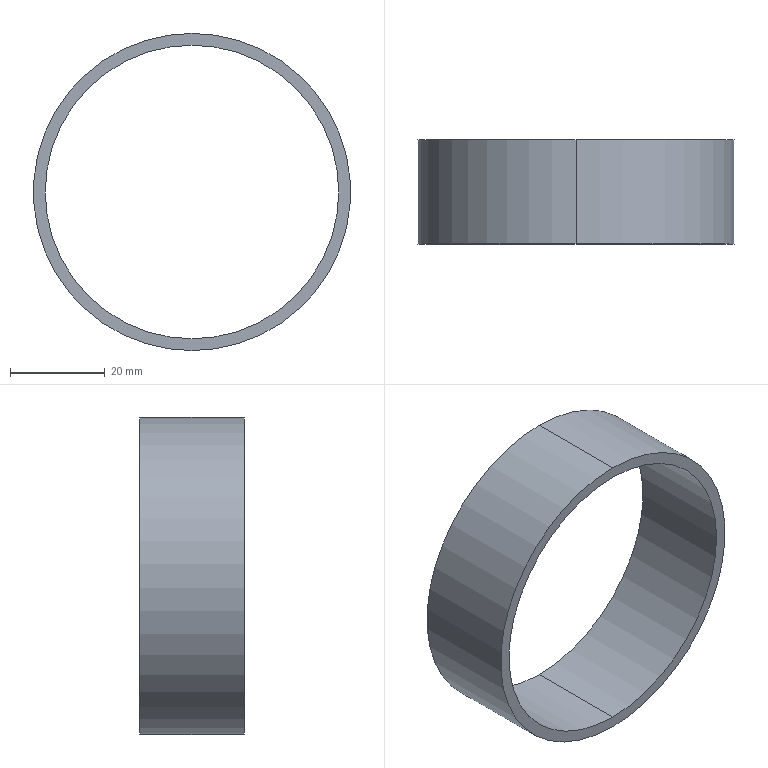Part | SolidWorks | features BaseBody 1 | 1 solid | 6 faces | box 67 x 22 x 67 mm | volume 11145 mm3 | cylinder 4 | plane 2 | commonest cylinder face diameters 62 x2 67 x2
STEP:
#1=CARTESIAN_POINT('',(-2132.95,902.097,-1608.624));
#2=VERTEX_POINT('',#1);
#3=CARTESIAN_POINT('',(-2132.95,902.097,-1546.624));
#4=VERTEX_POINT('',#3);
#5=CARTESIAN_POINT('',(-2132.95,902.097,-1577.624));
#6=DIRECTION('',(0.,-1.,0.));
#7=DIRECTION('',(0.,0.,-1.));
#8=AXIS2_PLACEMENT_3D('',#5,#6,#7);
#9=CIRCLE('',#8,31.);
#10=EDGE_CURVE('',#2,#4,#9,.T.);
#11=ORIENTED_EDGE('',*,*,#10,.F.);
#12=CARTESIAN_POINT('',(-2132.95,902.097,-1577.624));
#13=DIRECTION('',(0.,-1.,0.));
#14=DIRECTION('',(0.,0.,1.));
#15=AXIS2_PLACEMENT_3D('',#12,#13,#14);
#16=CIRCLE('',#15,31.);
#17=EDGE_CURVE('',#4,#2,#16,.T.);
#18=ORIENTED_EDGE('',*,*,#17,.F.);
#19=EDGE_LOOP('',(#11,#18));
#20=FACE_BOUND('',#19,.T.);
#21=CARTESIAN_POINT('',(-2132.95,902.097,-1611.124));
#22=VERTEX_POINT('',#21);
#23=CARTESIAN_POINT('',(-2132.95,902.097,-1544.124));
#24=VERTEX_POINT('',#23);
#25=CARTESIAN_POINT('',(-2132.95,902.097,-1577.624));
#26=DIRECTION('',(0.,-1.,0.));
#27=DIRECTION('',(0.,0.,-1.));
#28=AXIS2_PLACEMENT_3D('',#25,#26,#27);
#29=CIRCLE('',#28,33.5);
#30=EDGE_CURVE('',#22,#24,#29,.T.);
#31=ORIENTED_EDGE('',*,*,#30,.T.);
#32=CARTESIAN_POINT('',(-2132.95,902.097,-1577.624));
#33=DIRECTION('',(0.,-1.,0.));
#34=DIRECTION('',(0.,0.,1.));
#35=AXIS2_PLACEMENT_3D('',#32,#33,#34);
#36=CIRCLE('',#35,33.5);
#37=EDGE_CURVE('',#24,#22,#36,.T.);
#38=ORIENTED_EDGE('',*,*,#37,.T.);
#39=EDGE_LOOP('',(#31,#38));
#40=FACE_OUTER_BOUND('',#39,.T.);
#41=CARTESIAN_POINT('',(-2169.8,902.097,-1540.774));
#42=DIRECTION('',(0.,-1.,0.));
#43=DIRECTION('',(0.,0.,-1.));
#44=AXIS2_PLACEMENT_3D('',#41,#42,#43);
#45=PLANE('',#44);
#46=ADVANCED_FACE('',(#20,#40),#45,.T.);
#47=CARTESIAN_POINT('',(-2132.95,924.097,-1546.624));
#48=VERTEX_POINT('',#47);
#49=CARTESIAN_POINT('',(-2132.95,902.097,-1546.624));
#50=DIRECTION('',(0.,1.,0.));
#51=VECTOR('',#50,1000.);
#52=LINE('',#49,#51);
#53=EDGE_CURVE('',#4,#48,#52,.T.);
#54=ORIENTED_EDGE('',*,*,#53,.T.);
#55=CARTESIAN_POINT('',(-2132.95,924.097,-1608.624));
#56=VERTEX_POINT('',#55);
#57=CARTESIAN_POINT('',(-2132.95,924.097,-1577.624));
#58=DIRECTION('',(0.,1.,0.));
#59=DIRECTION('',(0.,0.,1.));
#60=AXIS2_PLACEMENT_3D('',#57,#58,#59);
#61=CIRCLE('',#60,31.);
#62=EDGE_CURVE('',#48,#56,#61,.T.);
#63=ORIENTED_EDGE('',*,*,#62,.T.);
#64=CARTESIAN_POINT('',(-2132.95,924.097,-1608.624));
#65=DIRECTION('',(0.,-1.,0.));
#66=VECTOR('',#65,1000.);
#67=LINE('',#64,#66);
#68=EDGE_CURVE('',#56,#2,#67,.T.);
#69=ORIENTED_EDGE('',*,*,#68,.T.);
#70=ORIENTED_EDGE('',*,*,#10,.T.);
#71=EDGE_LOOP('',(#54,#63,#69,#70));
#72=FACE_OUTER_BOUND('',#71,.T.);
#73=CARTESIAN_POINT('',(-2132.95,925.197,-1577.624));
#74=DIRECTION('',(0.,-1.,0.));
#75=DIRECTION('',(-0.08716,0.,-0.9962));
#76=AXIS2_PLACEMENT_3D('',#73,#74,#75);
#77=CYLINDRICAL_SURFACE('',#76,31.);
#78=ADVANCED_FACE('',(#72),#77,.F.);
#79=ORIENTED_EDGE('',*,*,#62,.F.);
#80=CARTESIAN_POINT('',(-2132.95,924.097,-1577.624));
#81=DIRECTION('',(0.,1.,0.));
#82=DIRECTION('',(0.,0.,-1.));
#83=AXIS2_PLACEMENT_3D('',#80,#81,#82);
#84=CIRCLE('',#83,31.);
#85=EDGE_CURVE('',#56,#48,#84,.T.);
#86=ORIENTED_EDGE('',*,*,#85,.F.);
#87=EDGE_LOOP('',(#79,#86));
#88=FACE_BOUND('',#87,.T.);
#89=CARTESIAN_POINT('',(-2132.95,924.097,-1544.124));
#90=VERTEX_POINT('',#89);
#91=CARTESIAN_POINT('',(-2132.95,924.097,-1611.124));
#92=VERTEX_POINT('',#91);
#93=CARTESIAN_POINT('',(-2132.95,924.097,-1577.624));
#94=DIRECTION('',(0.,1.,0.));
#95=DIRECTION('',(0.,0.,1.));
#96=AXIS2_PLACEMENT_3D('',#93,#94,#95);
#97=CIRCLE('',#96,33.5);
#98=EDGE_CURVE('',#90,#92,#97,.T.);
#99=ORIENTED_EDGE('',*,*,#98,.T.);
#100=CARTESIAN_POINT('',(-2132.95,924.097,-1577.624));
#101=DIRECTION('',(0.,1.,0.));
#102=DIRECTION('',(0.,0.,-1.));
#103=AXIS2_PLACEMENT_3D('',#100,#101,#102);
#104=CIRCLE('',#103,33.5);
#105=EDGE_CURVE('',#92,#90,#104,.T.);
#106=ORIENTED_EDGE('',*,*,#105,.T.);
#107=EDGE_LOOP('',(#99,#106));
#108=FACE_OUTER_BOUND('',#107,.T.);
#109=CARTESIAN_POINT('',(-2169.8,924.097,-1614.474));
#110=DIRECTION('',(0.,1.,0.));
#111=DIRECTION('',(1.,0.,0.));
#112=AXIS2_PLACEMENT_3D('',#109,#110,#111);
#113=PLANE('',#112);
#114=ADVANCED_FACE('',(#88,#108),#113,.T.);
#115=CARTESIAN_POINT('',(-2132.95,902.097,-1544.124));
#116=DIRECTION('',(0.,1.,0.));
#117=VECTOR('',#116,1000.);
#118=LINE('',#115,#117);
#119=EDGE_CURVE('',#24,#90,#118,.T.);
#120=ORIENTED_EDGE('',*,*,#119,.T.);
#121=ORIENTED_EDGE('',*,*,#105,.F.);
#122=CARTESIAN_POINT('',(-2132.95,924.097,-1611.124));
#123=DIRECTION('',(0.,-1.,0.));
#124=VECTOR('',#123,1000.);
#125=LINE('',#122,#124);
#126=EDGE_CURVE('',#92,#22,#125,.T.);
#127=ORIENTED_EDGE('',*,*,#126,.T.);
#128=ORIENTED_EDGE('',*,*,#37,.F.);
#129=EDGE_LOOP('',(#120,#121,#127,#128));
#130=FACE_OUTER_BOUND('',#129,.T.);
#131=CARTESIAN_POINT('',(-2132.95,900.997,-1577.624));
#132=DIRECTION('',(0.,-1.,0.));
#133=DIRECTION('',(0.08716,0.,0.9962));
#134=AXIS2_PLACEMENT_3D('',#131,#132,#133);
#135=CYLINDRICAL_SURFACE('',#134,33.5);
#136=ADVANCED_FACE('',(#130),#135,.T.);
#137=ORIENTED_EDGE('',*,*,#119,.F.);
#138=ORIENTED_EDGE('',*,*,#30,.F.);
#139=ORIENTED_EDGE('',*,*,#126,.F.);
#140=ORIENTED_EDGE('',*,*,#98,.F.);
#141=EDGE_LOOP('',(#137,#138,#139,#140));
#142=FACE_OUTER_BOUND('',#141,.T.);
#143=CARTESIAN_POINT('',(-2132.95,900.997,-1577.624));
#144=DIRECTION('',(0.,-1.,0.));
#145=DIRECTION('',(-0.08716,0.,-0.9962));
#146=AXIS2_PLACEMENT_3D('',#143,#144,#145);
#147=CYLINDRICAL_SURFACE('',#146,33.5);
#148=ADVANCED_FACE('',(#142),#147,.T.);
#149=ORIENTED_EDGE('',*,*,#53,.F.);
#150=ORIENTED_EDGE('',*,*,#17,.T.);
#151=ORIENTED_EDGE('',*,*,#68,.F.);
#152=ORIENTED_EDGE('',*,*,#85,.T.);
#153=EDGE_LOOP('',(#149,#150,#151,#152));
#154=FACE_OUTER_BOUND('',#153,.T.);
#155=CARTESIAN_POINT('',(-2132.95,925.197,-1577.624));
#156=DIRECTION('',(0.,-1.,0.));
#157=DIRECTION('',(0.08716,0.,0.9962));
#158=AXIS2_PLACEMENT_3D('',#155,#156,#157);
#159=CYLINDRICAL_SURFACE('',#158,31.);
#160=ADVANCED_FACE('',(#154),#159,.F.);
#161=CLOSED_SHELL('',(#46,#78,#114,#136,#148,#160));
#162=MANIFOLD_SOLID_BREP('',#161);
#163=CARTESIAN_POINT('',(0.,0.,0.));
#164=DIRECTION('',(0.,0.,1.));
#165=DIRECTION('',(1.,0.,0.));
#166=AXIS2_PLACEMENT_3D('',#163,#164,#165);
#167=(LENGTH_UNIT()NAMED_UNIT(*)SI_UNIT(.MILLI.,.METRE.));
#168=UNCERTAINTY_MEASURE_WITH_UNIT(LENGTH_MEASURE(0.00001),#167,'','');
#169=(NAMED_UNIT(*)PLANE_ANGLE_UNIT()SI_UNIT($,.RADIAN.));
#170=(NAMED_UNIT(*)SI_UNIT($,.STERADIAN.)SOLID_ANGLE_UNIT());
#171=(GEOMETRIC_REPRESENTATION_CONTEXT(3)GLOBAL_UNCERTAINTY_ASSIGNED_CONTEXT((#168))GLOBAL_UNIT_ASSIGNED_CONTEXT((#167,#169,#170))REPRESENTATION_CONTEXT('',''));
#172=ADVANCED_BREP_SHAPE_REPRESENTATION('',(#162,#166),#171);